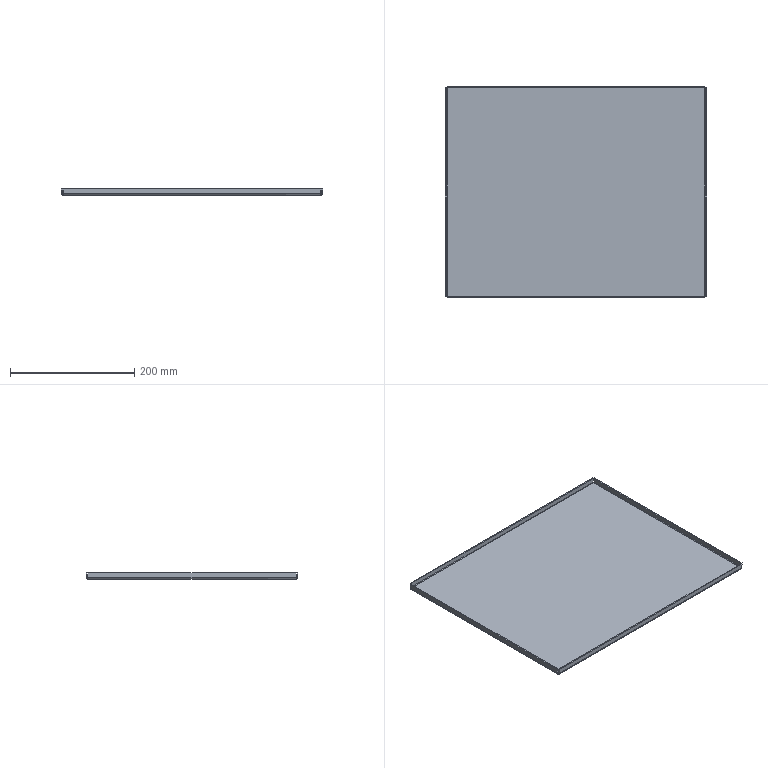Part | SolidWorks | features BaseBody 1 | 1 solid | 38 faces | box 420 x 340 x 10 mm | volume 307281 mm3 | plane 22 | cylinder 8 | spline 8 | commonest cylinder face diameters 1.473 x4 5.473 x4
STEP:
#1=CARTESIAN_POINT('',(-207.263,-167.263,-2.));
#2=VERTEX_POINT('',#1);
#3=CARTESIAN_POINT('',(-207.263,167.263,-2.));
#4=VERTEX_POINT('',#3);
#5=CARTESIAN_POINT('',(-207.263,0.,-2.));
#6=DIRECTION('',(0.,1.,0.));
#7=VECTOR('',#6,1000.);
#8=LINE('',#5,#7);
#9=EDGE_CURVE('',#2,#4,#8,.T.);
#10=ORIENTED_EDGE('',*,*,#9,.T.);
#11=CARTESIAN_POINT('',(207.263,167.263,-2.));
#12=VERTEX_POINT('',#11);
#13=CARTESIAN_POINT('',(0.,167.263,-2.));
#14=DIRECTION('',(1.,0.,0.));
#15=VECTOR('',#14,1000.);
#16=LINE('',#13,#15);
#17=EDGE_CURVE('',#4,#12,#16,.T.);
#18=ORIENTED_EDGE('',*,*,#17,.T.);
#19=CARTESIAN_POINT('',(207.263,-167.263,-2.));
#20=VERTEX_POINT('',#19);
#21=CARTESIAN_POINT('',(207.263,0.,-2.));
#22=DIRECTION('',(0.,-1.,0.));
#23=VECTOR('',#22,1000.);
#24=LINE('',#21,#23);
#25=EDGE_CURVE('',#12,#20,#24,.T.);
#26=ORIENTED_EDGE('',*,*,#25,.T.);
#27=CARTESIAN_POINT('',(0.,-167.263,-2.));
#28=DIRECTION('',(-1.,0.,0.));
#29=VECTOR('',#28,1000.);
#30=LINE('',#27,#29);
#31=EDGE_CURVE('',#20,#2,#30,.T.);
#32=ORIENTED_EDGE('',*,*,#31,.T.);
#33=EDGE_LOOP('',(#10,#18,#26,#32));
#34=FACE_OUTER_BOUND('',#33,.T.);
#35=CARTESIAN_POINT('',(207.263,-167.263,-2.));
#36=DIRECTION('',(0.,0.,-1.));
#37=DIRECTION('',(-1.,0.,0.));
#38=AXIS2_PLACEMENT_3D('',#35,#36,#37);
#39=PLANE('',#38);
#40=ADVANCED_FACE('',(#34),#39,.T.);
#41=CARTESIAN_POINT('',(-207.293,170.,0.7366));
#42=VERTEX_POINT('',#41);
#43=CARTESIAN_POINT('',(-207.293,170.,0.7366));
#44=CARTESIAN_POINT('',(-207.29,170.,0.3784));
#45=CARTESIAN_POINT('',(-207.288,169.929,0.0203));
#46=CARTESIAN_POINT('',(-207.283,169.655,-0.6416));
#47=CARTESIAN_POINT('',(-207.281,169.452,-0.9452));
#48=CARTESIAN_POINT('',(-207.276,168.945,-1.452));
#49=CARTESIAN_POINT('',(-207.273,168.642,-1.655));
#50=CARTESIAN_POINT('',(-207.268,167.98,-1.929));
#51=CARTESIAN_POINT('',(-207.266,167.622,-2.));
#52=CARTESIAN_POINT('',(-207.263,167.263,-2.));
#53=B_SPLINE_CURVE_WITH_KNOTS('',3,(#43,#44,#45,#46,#47,#48,#49,#50,#51,#52),.UNSPECIFIED.,.F.,.F.,(4,2,2,2,4),(0.,0.25,0.5,0.75,1.),.UNSPECIFIED.);
#54=EDGE_CURVE('',#42,#4,#53,.T.);
#55=ORIENTED_EDGE('',*,*,#54,.F.);
#56=CARTESIAN_POINT('',(207.293,170.,0.7366));
#57=VERTEX_POINT('',#56);
#58=CARTESIAN_POINT('',(0.,170.,0.7366));
#59=DIRECTION('',(-1.,0.,0.));
#60=VECTOR('',#59,1000.);
#61=LINE('',#58,#60);
#62=EDGE_CURVE('',#57,#42,#61,.T.);
#63=ORIENTED_EDGE('',*,*,#62,.F.);
#64=CARTESIAN_POINT('',(207.263,167.263,-2.));
#65=CARTESIAN_POINT('',(207.266,167.622,-2.));
#66=CARTESIAN_POINT('',(207.268,167.98,-1.929));
#67=CARTESIAN_POINT('',(207.273,168.642,-1.655));
#68=CARTESIAN_POINT('',(207.276,168.945,-1.452));
#69=CARTESIAN_POINT('',(207.281,169.452,-0.9452));
#70=CARTESIAN_POINT('',(207.283,169.655,-0.6416));
#71=CARTESIAN_POINT('',(207.288,169.929,0.0203));
#72=CARTESIAN_POINT('',(207.29,170.,0.3784));
#73=CARTESIAN_POINT('',(207.293,170.,0.7366));
#74=B_SPLINE_CURVE_WITH_KNOTS('',3,(#64,#65,#66,#67,#68,#69,#70,#71,#72,#73),.UNSPECIFIED.,.F.,.F.,(4,2,2,2,4),(0.,0.25,0.5,0.75,1.),.UNSPECIFIED.);
#75=EDGE_CURVE('',#12,#57,#74,.T.);
#76=ORIENTED_EDGE('',*,*,#75,.F.);
#77=ORIENTED_EDGE('',*,*,#17,.F.);
#78=EDGE_LOOP('',(#55,#63,#76,#77));
#79=FACE_OUTER_BOUND('',#78,.T.);
#80=CARTESIAN_POINT('',(209.78,167.263,0.7366));
#81=DIRECTION('',(-1.,0.,0.));
#82=DIRECTION('',(0.,0.,1.));
#83=AXIS2_PLACEMENT_3D('',#80,#81,#82);
#84=CYLINDRICAL_SURFACE('',#83,2.737);
#85=ADVANCED_FACE('',(#79),#84,.T.);
#86=CARTESIAN_POINT('',(-210.,-167.293,0.7366));
#87=VERTEX_POINT('',#86);
#88=CARTESIAN_POINT('',(-210.,-167.293,0.7366));
#89=CARTESIAN_POINT('',(-210.,-167.29,0.3784));
#90=CARTESIAN_POINT('',(-209.929,-167.288,0.0203));
#91=CARTESIAN_POINT('',(-209.655,-167.283,-0.6416));
#92=CARTESIAN_POINT('',(-209.452,-167.281,-0.9452));
#93=CARTESIAN_POINT('',(-208.945,-167.276,-1.452));
#94=CARTESIAN_POINT('',(-208.642,-167.273,-1.655));
#95=CARTESIAN_POINT('',(-207.98,-167.268,-1.929));
#96=CARTESIAN_POINT('',(-207.622,-167.266,-2.));
#97=CARTESIAN_POINT('',(-207.263,-167.263,-2.));
#98=B_SPLINE_CURVE_WITH_KNOTS('',3,(#88,#89,#90,#91,#92,#93,#94,#95,#96,#97),.UNSPECIFIED.,.F.,.F.,(4,2,2,2,4),(0.,0.25,0.5,0.75,1.),.UNSPECIFIED.);
#99=EDGE_CURVE('',#87,#2,#98,.T.);
#100=ORIENTED_EDGE('',*,*,#99,.F.);
#101=CARTESIAN_POINT('',(-210.,167.293,0.7366));
#102=VERTEX_POINT('',#101);
#103=CARTESIAN_POINT('',(-210.,0.,0.7366));
#104=DIRECTION('',(0.,-1.,0.));
#105=VECTOR('',#104,1000.);
#106=LINE('',#103,#105);
#107=EDGE_CURVE('',#102,#87,#106,.T.);
#108=ORIENTED_EDGE('',*,*,#107,.F.);
#109=CARTESIAN_POINT('',(-207.263,167.263,-2.));
#110=CARTESIAN_POINT('',(-207.622,167.266,-2.));
#111=CARTESIAN_POINT('',(-207.98,167.268,-1.929));
#112=CARTESIAN_POINT('',(-208.642,167.273,-1.655));
#113=CARTESIAN_POINT('',(-208.945,167.276,-1.452));
#114=CARTESIAN_POINT('',(-209.452,167.281,-0.9452));
#115=CARTESIAN_POINT('',(-209.655,167.283,-0.6416));
#116=CARTESIAN_POINT('',(-209.929,167.288,0.0203));
#117=CARTESIAN_POINT('',(-210.,167.29,0.3784));
#118=CARTESIAN_POINT('',(-210.,167.293,0.7366));
#119=B_SPLINE_CURVE_WITH_KNOTS('',3,(#109,#110,#111,#112,#113,#114,#115,#116,#117,#118),.UNSPECIFIED.,.F.,.F.,(4,2,2,2,4),(0.,0.25,0.5,0.75,1.),.UNSPECIFIED.);
#120=EDGE_CURVE('',#4,#102,#119,.T.);
#121=ORIENTED_EDGE('',*,*,#120,.F.);
#122=ORIENTED_EDGE('',*,*,#9,.F.);
#123=EDGE_LOOP('',(#100,#108,#121,#122));
#124=FACE_OUTER_BOUND('',#123,.T.);
#125=CARTESIAN_POINT('',(-207.263,169.3,0.7366));
#126=DIRECTION('',(0.,-1.,0.));
#127=DIRECTION('',(0.,0.,-1.));
#128=AXIS2_PLACEMENT_3D('',#125,#126,#127);
#129=CYLINDRICAL_SURFACE('',#128,2.737);
#130=ADVANCED_FACE('',(#124),#129,.T.);
#131=CARTESIAN_POINT('',(207.293,-170.,0.7366));
#132=VERTEX_POINT('',#131);
#133=CARTESIAN_POINT('',(207.293,-170.,0.7366));
#134=CARTESIAN_POINT('',(207.29,-170.,0.3784));
#135=CARTESIAN_POINT('',(207.288,-169.929,0.0203));
#136=CARTESIAN_POINT('',(207.283,-169.655,-0.6416));
#137=CARTESIAN_POINT('',(207.281,-169.452,-0.9452));
#138=CARTESIAN_POINT('',(207.276,-168.945,-1.452));
#139=CARTESIAN_POINT('',(207.273,-168.642,-1.655));
#140=CARTESIAN_POINT('',(207.268,-167.98,-1.929));
#141=CARTESIAN_POINT('',(207.266,-167.622,-2.));
#142=CARTESIAN_POINT('',(207.263,-167.263,-2.));
#143=B_SPLINE_CURVE_WITH_KNOTS('',3,(#133,#134,#135,#136,#137,#138,#139,#140,#141,#142),.UNSPECIFIED.,.F.,.F.,(4,2,2,2,4),(0.,0.25,0.5,0.75,1.),.UNSPECIFIED.);
#144=EDGE_CURVE('',#132,#20,#143,.T.);
#145=ORIENTED_EDGE('',*,*,#144,.F.);
#146=CARTESIAN_POINT('',(-207.293,-170.,0.7366));
#147=VERTEX_POINT('',#146);
#148=CARTESIAN_POINT('',(0.,-170.,0.7366));
#149=DIRECTION('',(1.,0.,0.));
#150=VECTOR('',#149,1000.);
#151=LINE('',#148,#150);
#152=EDGE_CURVE('',#147,#132,#151,.T.);
#153=ORIENTED_EDGE('',*,*,#152,.F.);
#154=CARTESIAN_POINT('',(-207.263,-167.263,-2.));
#155=CARTESIAN_POINT('',(-207.266,-167.622,-2.));
#156=CARTESIAN_POINT('',(-207.268,-167.98,-1.929));
#157=CARTESIAN_POINT('',(-207.273,-168.642,-1.655));
#158=CARTESIAN_POINT('',(-207.276,-168.945,-1.452));
#159=CARTESIAN_POINT('',(-207.281,-169.452,-0.9452));
#160=CARTESIAN_POINT('',(-207.283,-169.655,-0.6416));
#161=CARTESIAN_POINT('',(-207.288,-169.929,0.0203));
#162=CARTESIAN_POINT('',(-207.29,-170.,0.3784));
#163=CARTESIAN_POINT('',(-207.293,-170.,0.7366));
#164=B_SPLINE_CURVE_WITH_KNOTS('',3,(#154,#155,#156,#157,#158,#159,#160,#161,#162,#163),.UNSPECIFIED.,.F.,.F.,(4,2,2,2,4),(0.,0.25,0.5,0.75,1.),.UNSPECIFIED.);
#165=EDGE_CURVE('',#2,#147,#164,.T.);
#166=ORIENTED_EDGE('',*,*,#165,.F.);
#167=ORIENTED_EDGE('',*,*,#31,.F.);
#168=EDGE_LOOP('',(#145,#153,#166,#167));
#169=FACE_OUTER_BOUND('',#168,.T.);
#170=CARTESIAN_POINT('',(-209.78,-167.263,0.7366));
#171=DIRECTION('',(1.,0.,0.));
#172=DIRECTION('',(0.,0.,-1.));
#173=AXIS2_PLACEMENT_3D('',#170,#171,#172);
#174=CYLINDRICAL_SURFACE('',#173,2.737);
#175=ADVANCED_FACE('',(#169),#174,.T.);
#176=CARTESIAN_POINT('',(210.,167.293,0.7366));
#177=VERTEX_POINT('',#176);
#178=CARTESIAN_POINT('',(210.,167.293,0.7366));
#179=CARTESIAN_POINT('',(210.,167.29,0.3784));
#180=CARTESIAN_POINT('',(209.929,167.288,0.0203));
#181=CARTESIAN_POINT('',(209.655,167.283,-0.6416));
#182=CARTESIAN_POINT('',(209.452,167.281,-0.9452));
#183=CARTESIAN_POINT('',(208.945,167.276,-1.452));
#184=CARTESIAN_POINT('',(208.642,167.273,-1.655));
#185=CARTESIAN_POINT('',(207.98,167.268,-1.929));
#186=CARTESIAN_POINT('',(207.622,167.266,-2.));
#187=CARTESIAN_POINT('',(207.263,167.263,-2.));
#188=B_SPLINE_CURVE_WITH_KNOTS('',3,(#178,#179,#180,#181,#182,#183,#184,#185,#186,#187),.UNSPECIFIED.,.F.,.F.,(4,2,2,2,4),(0.,0.25,0.5,0.75,1.),.UNSPECIFIED.);
#189=EDGE_CURVE('',#177,#12,#188,.T.);
#190=ORIENTED_EDGE('',*,*,#189,.F.);
#191=CARTESIAN_POINT('',(210.,-167.293,0.7366));
#192=VERTEX_POINT('',#191);
#193=CARTESIAN_POINT('',(210.,0.,0.7366));
#194=DIRECTION('',(0.,1.,0.));
#195=VECTOR('',#194,1000.);
#196=LINE('',#193,#195);
#197=EDGE_CURVE('',#192,#177,#196,.T.);
#198=ORIENTED_EDGE('',*,*,#197,.F.);
#199=CARTESIAN_POINT('',(207.263,-167.263,-2.));
#200=CARTESIAN_POINT('',(207.622,-167.266,-2.));
#201=CARTESIAN_POINT('',(207.98,-167.268,-1.929));
#202=CARTESIAN_POINT('',(208.642,-167.273,-1.655));
#203=CARTESIAN_POINT('',(208.945,-167.276,-1.452));
#204=CARTESIAN_POINT('',(209.452,-167.281,-0.9452));
#205=CARTESIAN_POINT('',(209.655,-167.283,-0.6416));
#206=CARTESIAN_POINT('',(209.929,-167.288,0.0203));
#207=CARTESIAN_POINT('',(210.,-167.29,0.3784));
#208=CARTESIAN_POINT('',(210.,-167.293,0.7366));
#209=B_SPLINE_CURVE_WITH_KNOTS('',3,(#199,#200,#201,#202,#203,#204,#205,#206,#207,#208),.UNSPECIFIED.,.F.,.F.,(4,2,2,2,4),(0.,0.25,0.5,0.75,1.),.UNSPECIFIED.);
#210=EDGE_CURVE('',#20,#192,#209,.T.);
#211=ORIENTED_EDGE('',*,*,#210,.F.);
#212=ORIENTED_EDGE('',*,*,#25,.F.);
#213=EDGE_LOOP('',(#190,#198,#211,#212));
#214=FACE_OUTER_BOUND('',#213,.T.);
#215=CARTESIAN_POINT('',(207.263,-169.3,0.7366));
#216=DIRECTION('',(0.,1.,0.));
#217=DIRECTION('',(0.,0.,1.));
#218=AXIS2_PLACEMENT_3D('',#215,#216,#217);
#219=CYLINDRICAL_SURFACE('',#218,2.737);
#220=ADVANCED_FACE('',(#214),#219,.T.);
#221=CARTESIAN_POINT('',(-207.293,168.,0.7366));
#222=VERTEX_POINT('',#221);
#223=CARTESIAN_POINT('',(-207.293,169.,0.7366));
#224=DIRECTION('',(0.,-1.,0.));
#225=VECTOR('',#224,1000.);
#226=LINE('',#223,#225);
#227=EDGE_CURVE('',#42,#222,#226,.T.);
#228=ORIENTED_EDGE('',*,*,#227,.F.);
#229=ORIENTED_EDGE('',*,*,#54,.T.);
#230=CARTESIAN_POINT('',(-207.263,167.263,0.));
#231=VERTEX_POINT('',#230);
#232=CARTESIAN_POINT('',(-207.263,167.263,-1.));
#233=DIRECTION('',(0.,0.,-1.));
#234=VECTOR('',#233,1000.);
#235=LINE('',#232,#234);
#236=EDGE_CURVE('',#231,#4,#235,.T.);
#237=ORIENTED_EDGE('',*,*,#236,.F.);
#238=CARTESIAN_POINT('',(-207.293,168.,0.7366));
#239=CARTESIAN_POINT('',(-207.288,168.,0.5438));
#240=CARTESIAN_POINT('',(-207.283,167.921,0.3521));
#241=CARTESIAN_POINT('',(-207.273,167.648,0.07939));
#242=CARTESIAN_POINT('',(-207.268,167.456,0.));
#243=CARTESIAN_POINT('',(-207.263,167.263,0.));
#244=B_SPLINE_CURVE_WITH_KNOTS('',3,(#238,#239,#240,#241,#242,#243),.UNSPECIFIED.,.F.,.F.,(4,2,4),(0.,0.5,1.),.UNSPECIFIED.);
#245=EDGE_CURVE('',#222,#231,#244,.T.);
#246=ORIENTED_EDGE('',*,*,#245,.F.);
#247=EDGE_LOOP('',(#228,#229,#237,#246));
#248=FACE_OUTER_BOUND('',#247,.T.);
#249=CARTESIAN_POINT('',(-207.293,170.012,0.7366));
#250=CARTESIAN_POINT('',(-207.29,170.012,0.3767));
#251=CARTESIAN_POINT('',(-207.288,169.941,0.01711));
#252=CARTESIAN_POINT('',(-207.283,169.665,-0.6477));
#253=CARTESIAN_POINT('',(-207.281,169.462,-0.9527));
#254=CARTESIAN_POINT('',(-207.276,168.953,-1.462));
#255=CARTESIAN_POINT('',(-207.273,168.648,-1.665));
#256=CARTESIAN_POINT('',(-207.268,167.983,-1.941));
#257=CARTESIAN_POINT('',(-207.266,167.623,-2.012));
#258=CARTESIAN_POINT('',(-207.263,167.263,-2.012));
#259=CARTESIAN_POINT('',(-207.293,170.,0.7366));
#260=CARTESIAN_POINT('',(-207.29,170.,0.3783));
#261=CARTESIAN_POINT('',(-207.288,169.929,0.0203));
#262=CARTESIAN_POINT('',(-207.283,169.655,-0.6416));
#263=CARTESIAN_POINT('',(-207.281,169.452,-0.9452));
#264=CARTESIAN_POINT('',(-207.276,168.945,-1.452));
#265=CARTESIAN_POINT('',(-207.273,168.642,-1.655));
#266=CARTESIAN_POINT('',(-207.268,167.98,-1.929));
#267=CARTESIAN_POINT('',(-207.266,167.622,-2.));
#268=CARTESIAN_POINT('',(-207.263,167.263,-2.));
#269=CARTESIAN_POINT('',(-207.293,168.,0.7366));
#270=CARTESIAN_POINT('',(-207.29,168.,0.6402));
#271=CARTESIAN_POINT('',(-207.288,167.981,0.5438));
#272=CARTESIAN_POINT('',(-207.283,167.907,0.3656));
#273=CARTESIAN_POINT('',(-207.281,167.852,0.2839));
#274=CARTESIAN_POINT('',(-207.276,167.716,0.1476));
#275=CARTESIAN_POINT('',(-207.273,167.634,0.09297));
#276=CARTESIAN_POINT('',(-207.268,167.456,0.01917));
#277=CARTESIAN_POINT('',(-207.266,167.36,0.));
#278=CARTESIAN_POINT('',(-207.263,167.263,0.));
#279=CARTESIAN_POINT('',(-207.293,167.988,0.7366));
#280=CARTESIAN_POINT('',(-207.29,167.988,0.6417));
#281=CARTESIAN_POINT('',(-207.288,167.969,0.5469));
#282=CARTESIAN_POINT('',(-207.283,167.897,0.3717));
#283=CARTESIAN_POINT('',(-207.281,167.843,0.2913));
#284=CARTESIAN_POINT('',(-207.276,167.709,0.1572));
#285=CARTESIAN_POINT('',(-207.273,167.628,0.1035));
#286=CARTESIAN_POINT('',(-207.268,167.453,0.03088));
#287=CARTESIAN_POINT('',(-207.266,167.358,0.01202));
#288=CARTESIAN_POINT('',(-207.263,167.263,0.01202));
#289=B_SPLINE_SURFACE_WITH_KNOTS('',1,3,((#249,#250,#251,#252,#253,#254,#255,#256,#257,#258),(#259,#260,#261,#262,#263,#264,#265,#266,#267,#268),(#269,#270,#271,#272,#273,#274,#275,#276,#277,#278),(#279,#280,#281,#282,#283,#284,#285,#286,#287,#288)),.UNSPECIFIED.,.F.,.F.,.F.,(2,1,1,2),(4,2,2,2,4),(-0.006096,0.,1.,1.006),(0.,0.25,0.5,0.75,1.),.UNSPECIFIED.);
#290=ADVANCED_FACE('',(#248),#289,.F.);
#291=CARTESIAN_POINT('',(-207.293,170.,8.));
#292=VERTEX_POINT('',#291);
#293=CARTESIAN_POINT('',(-207.293,170.,4.368));
#294=DIRECTION('',(0.,0.,-1.));
#295=VECTOR('',#294,1000.);
#296=LINE('',#293,#295);
#297=EDGE_CURVE('',#292,#42,#296,.T.);
#298=ORIENTED_EDGE('',*,*,#297,.F.);
#299=CARTESIAN_POINT('',(207.293,170.,8.));
#300=VERTEX_POINT('',#299);
#301=CARTESIAN_POINT('',(0.,170.,8.));
#302=DIRECTION('',(-1.,0.,0.));
#303=VECTOR('',#302,1000.);
#304=LINE('',#301,#303);
#305=EDGE_CURVE('',#300,#292,#304,.T.);
#306=ORIENTED_EDGE('',*,*,#305,.F.);
#307=CARTESIAN_POINT('',(207.293,170.,4.368));
#308=DIRECTION('',(0.,0.,1.));
#309=VECTOR('',#308,1000.);
#310=LINE('',#307,#309);
#311=EDGE_CURVE('',#57,#300,#310,.T.);
#312=ORIENTED_EDGE('',*,*,#311,.F.);
#313=ORIENTED_EDGE('',*,*,#62,.T.);
#314=EDGE_LOOP('',(#298,#306,#312,#313));
#315=FACE_OUTER_BOUND('',#314,.T.);
#316=CARTESIAN_POINT('',(-207.293,170.,8.));
#317=DIRECTION('',(0.,-1.,0.));
#318=DIRECTION('',(0.,0.,-1.));
#319=AXIS2_PLACEMENT_3D('',#316,#317,#318);
#320=PLANE('',#319);
#321=ADVANCED_FACE('',(#315),#320,.F.);
#322=CARTESIAN_POINT('',(207.263,167.263,0.));
#323=VERTEX_POINT('',#322);
#324=CARTESIAN_POINT('',(207.293,168.,0.7366));
#325=VERTEX_POINT('',#324);
#326=CARTESIAN_POINT('',(207.263,167.263,0.));
#327=CARTESIAN_POINT('',(207.268,167.456,0.));
#328=CARTESIAN_POINT('',(207.273,167.648,0.07939));
#329=CARTESIAN_POINT('',(207.283,167.921,0.3521));
#330=CARTESIAN_POINT('',(207.288,168.,0.5438));
#331=CARTESIAN_POINT('',(207.293,168.,0.7366));
#332=B_SPLINE_CURVE_WITH_KNOTS('',3,(#326,#327,#328,#329,#330,#331),.UNSPECIFIED.,.F.,.F.,(4,2,4),(0.,0.5,1.),.UNSPECIFIED.);
#333=EDGE_CURVE('',#323,#325,#332,.T.);
#334=ORIENTED_EDGE('',*,*,#333,.F.);
#335=CARTESIAN_POINT('',(207.263,167.263,-1.));
#336=DIRECTION('',(0.,0.,1.));
#337=VECTOR('',#336,1000.);
#338=LINE('',#335,#337);
#339=EDGE_CURVE('',#12,#323,#338,.T.);
#340=ORIENTED_EDGE('',*,*,#339,.F.);
#341=ORIENTED_EDGE('',*,*,#75,.T.);
#342=CARTESIAN_POINT('',(207.293,169.,0.7366));
#343=DIRECTION('',(0.,1.,0.));
#344=VECTOR('',#343,1000.);
#345=LINE('',#342,#344);
#346=EDGE_CURVE('',#325,#57,#345,.T.);
#347=ORIENTED_EDGE('',*,*,#346,.F.);
#348=EDGE_LOOP('',(#334,#340,#341,#347));
#349=FACE_OUTER_BOUND('',#348,.T.);
#350=CARTESIAN_POINT('',(207.263,167.263,-2.012));
#351=CARTESIAN_POINT('',(207.266,167.623,-2.012));
#352=CARTESIAN_POINT('',(207.268,167.983,-1.941));
#353=CARTESIAN_POINT('',(207.273,168.648,-1.665));
#354=CARTESIAN_POINT('',(207.276,168.953,-1.462));
#355=CARTESIAN_POINT('',(207.281,169.462,-0.9527));
#356=CARTESIAN_POINT('',(207.283,169.665,-0.6477));
#357=CARTESIAN_POINT('',(207.288,169.941,0.01711));
#358=CARTESIAN_POINT('',(207.29,170.012,0.3767));
#359=CARTESIAN_POINT('',(207.293,170.012,0.7366));
#360=CARTESIAN_POINT('',(207.263,167.263,-2.));
#361=CARTESIAN_POINT('',(207.266,167.622,-2.));
#362=CARTESIAN_POINT('',(207.268,167.98,-1.929));
#363=CARTESIAN_POINT('',(207.273,168.642,-1.655));
#364=CARTESIAN_POINT('',(207.276,168.945,-1.452));
#365=CARTESIAN_POINT('',(207.281,169.452,-0.9452));
#366=CARTESIAN_POINT('',(207.283,169.655,-0.6416));
#367=CARTESIAN_POINT('',(207.288,169.929,0.0203));
#368=CARTESIAN_POINT('',(207.29,170.,0.3783));
#369=CARTESIAN_POINT('',(207.293,170.,0.7366));
#370=CARTESIAN_POINT('',(207.263,167.263,0.));
#371=CARTESIAN_POINT('',(207.266,167.36,0.));
#372=CARTESIAN_POINT('',(207.268,167.456,0.01917));
#373=CARTESIAN_POINT('',(207.273,167.634,0.09297));
#374=CARTESIAN_POINT('',(207.276,167.716,0.1476));
#375=CARTESIAN_POINT('',(207.281,167.852,0.2839));
#376=CARTESIAN_POINT('',(207.283,167.907,0.3656));
#377=CARTESIAN_POINT('',(207.288,167.981,0.5438));
#378=CARTESIAN_POINT('',(207.29,168.,0.6402));
#379=CARTESIAN_POINT('',(207.293,168.,0.7366));
#380=CARTESIAN_POINT('',(207.263,167.263,0.01202));
#381=CARTESIAN_POINT('',(207.266,167.358,0.01202));
#382=CARTESIAN_POINT('',(207.268,167.453,0.03088));
#383=CARTESIAN_POINT('',(207.273,167.628,0.1035));
#384=CARTESIAN_POINT('',(207.276,167.709,0.1572));
#385=CARTESIAN_POINT('',(207.281,167.843,0.2913));
#386=CARTESIAN_POINT('',(207.283,167.897,0.3717));
#387=CARTESIAN_POINT('',(207.288,167.969,0.5469));
#388=CARTESIAN_POINT('',(207.29,167.988,0.6417));
#389=CARTESIAN_POINT('',(207.293,167.988,0.7366));
#390=B_SPLINE_SURFACE_WITH_KNOTS('',1,3,((#350,#351,#352,#353,#354,#355,#356,#357,#358,#359),(#360,#361,#362,#363,#364,#365,#366,#367,#368,#369),(#370,#371,#372,#373,#374,#375,#376,#377,#378,#379),(#380,#381,#382,#383,#384,#385,#386,#387,#388,#389)),.UNSPECIFIED.,.F.,.F.,.F.,(2,1,1,2),(4,2,2,2,4),(-0.006096,0.,1.,1.006),(0.,0.25,0.5,0.75,1.),.UNSPECIFIED.);
#391=ADVANCED_FACE('',(#349),#390,.F.);
#392=CARTESIAN_POINT('',(-208.,-167.293,0.7366));
#393=VERTEX_POINT('',#392);
#394=CARTESIAN_POINT('',(-209.,-167.293,0.7366));
#395=DIRECTION('',(1.,0.,0.));
#396=VECTOR('',#395,1000.);
#397=LINE('',#394,#396);
#398=EDGE_CURVE('',#87,#393,#397,.T.);
#399=ORIENTED_EDGE('',*,*,#398,.F.);
#400=ORIENTED_EDGE('',*,*,#99,.T.);
#401=CARTESIAN_POINT('',(-207.263,-167.263,0.));
#402=VERTEX_POINT('',#401);
#403=CARTESIAN_POINT('',(-207.263,-167.263,-1.));
#404=DIRECTION('',(0.,0.,-1.));
#405=VECTOR('',#404,1000.);
#406=LINE('',#403,#405);
#407=EDGE_CURVE('',#402,#2,#406,.T.);
#408=ORIENTED_EDGE('',*,*,#407,.F.);
#409=CARTESIAN_POINT('',(-208.,-167.293,0.7366));
#410=CARTESIAN_POINT('',(-208.,-167.288,0.5438));
#411=CARTESIAN_POINT('',(-207.921,-167.283,0.3521));
#412=CARTESIAN_POINT('',(-207.648,-167.273,0.07939));
#413=CARTESIAN_POINT('',(-207.456,-167.268,0.));
#414=CARTESIAN_POINT('',(-207.263,-167.263,0.));
#415=B_SPLINE_CURVE_WITH_KNOTS('',3,(#409,#410,#411,#412,#413,#414),.UNSPECIFIED.,.F.,.F.,(4,2,4),(0.,0.5,1.),.UNSPECIFIED.);
#416=EDGE_CURVE('',#393,#402,#415,.T.);
#417=ORIENTED_EDGE('',*,*,#416,.F.);
#418=EDGE_LOOP('',(#399,#400,#408,#417));
#419=FACE_OUTER_BOUND('',#418,.T.);
#420=CARTESIAN_POINT('',(-210.012,-167.293,0.7366));
#421=CARTESIAN_POINT('',(-210.012,-167.29,0.3767));
#422=CARTESIAN_POINT('',(-209.941,-167.288,0.01711));
#423=CARTESIAN_POINT('',(-209.665,-167.283,-0.6477));
#424=CARTESIAN_POINT('',(-209.462,-167.281,-0.9527));
#425=CARTESIAN_POINT('',(-208.953,-167.276,-1.462));
#426=CARTESIAN_POINT('',(-208.648,-167.273,-1.665));
#427=CARTESIAN_POINT('',(-207.983,-167.268,-1.941));
#428=CARTESIAN_POINT('',(-207.623,-167.266,-2.012));
#429=CARTESIAN_POINT('',(-207.263,-167.263,-2.012));
#430=CARTESIAN_POINT('',(-210.,-167.293,0.7366));
#431=CARTESIAN_POINT('',(-210.,-167.29,0.3783));
#432=CARTESIAN_POINT('',(-209.929,-167.288,0.0203));
#433=CARTESIAN_POINT('',(-209.655,-167.283,-0.6416));
#434=CARTESIAN_POINT('',(-209.452,-167.281,-0.9452));
#435=CARTESIAN_POINT('',(-208.945,-167.276,-1.452));
#436=CARTESIAN_POINT('',(-208.642,-167.273,-1.655));
#437=CARTESIAN_POINT('',(-207.98,-167.268,-1.929));
#438=CARTESIAN_POINT('',(-207.622,-167.266,-2.));
#439=CARTESIAN_POINT('',(-207.263,-167.263,-2.));
#440=CARTESIAN_POINT('',(-208.,-167.293,0.7366));
#441=CARTESIAN_POINT('',(-208.,-167.29,0.6402));
#442=CARTESIAN_POINT('',(-207.981,-167.288,0.5438));
#443=CARTESIAN_POINT('',(-207.907,-167.283,0.3656));
#444=CARTESIAN_POINT('',(-207.852,-167.281,0.2839));
#445=CARTESIAN_POINT('',(-207.716,-167.276,0.1476));
#446=CARTESIAN_POINT('',(-207.634,-167.273,0.09297));
#447=CARTESIAN_POINT('',(-207.456,-167.268,0.01917));
#448=CARTESIAN_POINT('',(-207.36,-167.266,0.));
#449=CARTESIAN_POINT('',(-207.263,-167.263,0.));
#450=CARTESIAN_POINT('',(-207.988,-167.293,0.7366));
#451=CARTESIAN_POINT('',(-207.988,-167.29,0.6417));
#452=CARTESIAN_POINT('',(-207.969,-167.288,0.5469));
#453=CARTESIAN_POINT('',(-207.897,-167.283,0.3717));
#454=CARTESIAN_POINT('',(-207.843,-167.281,0.2913));
#455=CARTESIAN_POINT('',(-207.709,-167.276,0.1572));
#456=CARTESIAN_POINT('',(-207.628,-167.273,0.1035));
#457=CARTESIAN_POINT('',(-207.453,-167.268,0.03088));
#458=CARTESIAN_POINT('',(-207.358,-167.266,0.01202));
#459=CARTESIAN_POINT('',(-207.263,-167.263,0.01202));
#460=B_SPLINE_SURFACE_WITH_KNOTS('',1,3,((#420,#421,#422,#423,#424,#425,#426,#427,#428,#429),(#430,#431,#432,#433,#434,#435,#436,#437,#438,#439),(#440,#441,#442,#443,#444,#445,#446,#447,#448,#449),(#450,#451,#452,#453,#454,#455,#456,#457,#458,#459)),.UNSPECIFIED.,.F.,.F.,.F.,(2,1,1,2),(4,2,2,2,4),(-0.006096,0.,1.,1.006),(0.,0.25,0.5,0.75,1.),.UNSPECIFIED.);
#461=ADVANCED_FACE('',(#419),#460,.F.);
#462=CARTESIAN_POINT('',(-210.,-167.293,8.));
#463=VERTEX_POINT('',#462);
#464=CARTESIAN_POINT('',(-210.,-167.293,4.368));
#465=DIRECTION('',(0.,0.,-1.));
#466=VECTOR('',#465,1000.);
#467=LINE('',#464,#466);
#468=EDGE_CURVE('',#463,#87,#467,.T.);
#469=ORIENTED_EDGE('',*,*,#468,.F.);
#470=CARTESIAN_POINT('',(-210.,167.293,8.));
#471=VERTEX_POINT('',#470);
#472=CARTESIAN_POINT('',(-210.,0.,8.));
#473=DIRECTION('',(0.,-1.,0.));
#474=VECTOR('',#473,1000.);
#475=LINE('',#472,#474);
#476=EDGE_CURVE('',#471,#463,#475,.T.);
#477=ORIENTED_EDGE('',*,*,#476,.F.);
#478=CARTESIAN_POINT('',(-210.,167.293,4.368));
#479=DIRECTION('',(0.,0.,1.));
#480=VECTOR('',#479,1000.);
#481=LINE('',#478,#480);
#482=EDGE_CURVE('',#102,#471,#481,.T.);
#483=ORIENTED_EDGE('',*,*,#482,.F.);
#484=ORIENTED_EDGE('',*,*,#107,.T.);
#485=EDGE_LOOP('',(#469,#477,#483,#484));
#486=FACE_OUTER_BOUND('',#485,.T.);
#487=CARTESIAN_POINT('',(-210.,-167.293,8.));
#488=DIRECTION('',(1.,0.,0.));
#489=DIRECTION('',(0.,0.,-1.));
#490=AXIS2_PLACEMENT_3D('',#487,#488,#489);
#491=PLANE('',#490);
#492=ADVANCED_FACE('',(#486),#491,.F.);
#493=CARTESIAN_POINT('',(-208.,167.293,0.7366));
#494=VERTEX_POINT('',#493);
#495=CARTESIAN_POINT('',(-207.263,167.263,0.));
#496=CARTESIAN_POINT('',(-207.456,167.268,0.));
#497=CARTESIAN_POINT('',(-207.648,167.273,0.07939));
#498=CARTESIAN_POINT('',(-207.921,167.283,0.3521));
#499=CARTESIAN_POINT('',(-208.,167.288,0.5438));
#500=CARTESIAN_POINT('',(-208.,167.293,0.7366));
#501=B_SPLINE_CURVE_WITH_KNOTS('',3,(#495,#496,#497,#498,#499,#500),.UNSPECIFIED.,.F.,.F.,(4,2,4),(0.,0.5,1.),.UNSPECIFIED.);
#502=EDGE_CURVE('',#231,#494,#501,.T.);
#503=ORIENTED_EDGE('',*,*,#502,.F.);
#504=ORIENTED_EDGE('',*,*,#236,.T.);
#505=ORIENTED_EDGE('',*,*,#120,.T.);
#506=CARTESIAN_POINT('',(-209.,167.293,0.7366));
#507=DIRECTION('',(-1.,0.,0.));
#508=VECTOR('',#507,1000.);
#509=LINE('',#506,#508);
#510=EDGE_CURVE('',#494,#102,#509,.T.);
#511=ORIENTED_EDGE('',*,*,#510,.F.);
#512=EDGE_LOOP('',(#503,#504,#505,#511));
#513=FACE_OUTER_BOUND('',#512,.T.);
#514=CARTESIAN_POINT('',(-207.263,167.263,-2.012));
#515=CARTESIAN_POINT('',(-207.623,167.266,-2.012));
#516=CARTESIAN_POINT('',(-207.983,167.268,-1.941));
#517=CARTESIAN_POINT('',(-208.648,167.273,-1.665));
#518=CARTESIAN_POINT('',(-208.953,167.276,-1.462));
#519=CARTESIAN_POINT('',(-209.462,167.281,-0.9527));
#520=CARTESIAN_POINT('',(-209.665,167.283,-0.6477));
#521=CARTESIAN_POINT('',(-209.941,167.288,0.01711));
#522=CARTESIAN_POINT('',(-210.012,167.29,0.3767));
#523=CARTESIAN_POINT('',(-210.012,167.293,0.7366));
#524=CARTESIAN_POINT('',(-207.263,167.263,-2.));
#525=CARTESIAN_POINT('',(-207.622,167.266,-2.));
#526=CARTESIAN_POINT('',(-207.98,167.268,-1.929));
#527=CARTESIAN_POINT('',(-208.642,167.273,-1.655));
#528=CARTESIAN_POINT('',(-208.945,167.276,-1.452));
#529=CARTESIAN_POINT('',(-209.452,167.281,-0.9452));
#530=CARTESIAN_POINT('',(-209.655,167.283,-0.6416));
#531=CARTESIAN_POINT('',(-209.929,167.288,0.0203));
#532=CARTESIAN_POINT('',(-210.,167.29,0.3783));
#533=CARTESIAN_POINT('',(-210.,167.293,0.7366));
#534=CARTESIAN_POINT('',(-207.263,167.263,0.));
#535=CARTESIAN_POINT('',(-207.36,167.266,0.));
#536=CARTESIAN_POINT('',(-207.456,167.268,0.01917));
#537=CARTESIAN_POINT('',(-207.634,167.273,0.09297));
#538=CARTESIAN_POINT('',(-207.716,167.276,0.1476));
#539=CARTESIAN_POINT('',(-207.852,167.281,0.2839));
#540=CARTESIAN_POINT('',(-207.907,167.283,0.3656));
#541=CARTESIAN_POINT('',(-207.981,167.288,0.5438));
#542=CARTESIAN_POINT('',(-208.,167.29,0.6402));
#543=CARTESIAN_POINT('',(-208.,167.293,0.7366));
#544=CARTESIAN_POINT('',(-207.263,167.263,0.01202));
#545=CARTESIAN_POINT('',(-207.358,167.266,0.01202));
#546=CARTESIAN_POINT('',(-207.453,167.268,0.03088));
#547=CARTESIAN_POINT('',(-207.628,167.273,0.1035));
#548=CARTESIAN_POINT('',(-207.709,167.276,0.1572));
#549=CARTESIAN_POINT('',(-207.843,167.281,0.2913));
#550=CARTESIAN_POINT('',(-207.897,167.283,0.3717));
#551=CARTESIAN_POINT('',(-207.969,167.288,0.5469));
#552=CARTESIAN_POINT('',(-207.988,167.29,0.6417));
#553=CARTESIAN_POINT('',(-207.988,167.293,0.7366));
#554=B_SPLINE_SURFACE_WITH_KNOTS('',1,3,((#514,#515,#516,#517,#518,#519,#520,#521,#522,#523),(#524,#525,#526,#527,#528,#529,#530,#531,#532,#533),(#534,#535,#536,#537,#538,#539,#540,#541,#542,#543),(#544,#545,#546,#547,#548,#549,#550,#551,#552,#553)),.UNSPECIFIED.,.F.,.F.,.F.,(2,1,1,2),(4,2,2,2,4),(-0.006096,0.,1.,1.006),(0.,0.25,0.5,0.75,1.),.UNSPECIFIED.);
#555=ADVANCED_FACE('',(#513),#554,.F.);
#556=CARTESIAN_POINT('',(207.293,-168.,0.7366));
#557=VERTEX_POINT('',#556);
#558=CARTESIAN_POINT('',(207.293,-169.,0.7366));
#559=DIRECTION('',(0.,1.,0.));
#560=VECTOR('',#559,1000.);
#561=LINE('',#558,#560);
#562=EDGE_CURVE('',#132,#557,#561,.T.);
#563=ORIENTED_EDGE('',*,*,#562,.F.);
#564=ORIENTED_EDGE('',*,*,#144,.T.);
#565=CARTESIAN_POINT('',(207.263,-167.263,0.));
#566=VERTEX_POINT('',#565);
#567=CARTESIAN_POINT('',(207.263,-167.263,-1.));
#568=DIRECTION('',(0.,0.,-1.));
#569=VECTOR('',#568,1000.);
#570=LINE('',#567,#569);
#571=EDGE_CURVE('',#566,#20,#570,.T.);
#572=ORIENTED_EDGE('',*,*,#571,.F.);
#573=CARTESIAN_POINT('',(207.293,-168.,0.7366));
#574=CARTESIAN_POINT('',(207.288,-168.,0.5438));
#575=CARTESIAN_POINT('',(207.283,-167.921,0.3521));
#576=CARTESIAN_POINT('',(207.273,-167.648,0.07939));
#577=CARTESIAN_POINT('',(207.268,-167.456,0.));
#578=CARTESIAN_POINT('',(207.263,-167.263,0.));
#579=B_SPLINE_CURVE_WITH_KNOTS('',3,(#573,#574,#575,#576,#577,#578),.UNSPECIFIED.,.F.,.F.,(4,2,4),(0.,0.5,1.),.UNSPECIFIED.);
#580=EDGE_CURVE('',#557,#566,#579,.T.);
#581=ORIENTED_EDGE('',*,*,#580,.F.);
#582=EDGE_LOOP('',(#563,#564,#572,#581));
#583=FACE_OUTER_BOUND('',#582,.T.);
#584=CARTESIAN_POINT('',(207.293,-170.012,0.7366));
#585=CARTESIAN_POINT('',(207.29,-170.012,0.3767));
#586=CARTESIAN_POINT('',(207.288,-169.941,0.01711));
#587=CARTESIAN_POINT('',(207.283,-169.665,-0.6477));
#588=CARTESIAN_POINT('',(207.281,-169.462,-0.9527));
#589=CARTESIAN_POINT('',(207.276,-168.953,-1.462));
#590=CARTESIAN_POINT('',(207.273,-168.648,-1.665));
#591=CARTESIAN_POINT('',(207.268,-167.983,-1.941));
#592=CARTESIAN_POINT('',(207.266,-167.623,-2.012));
#593=CARTESIAN_POINT('',(207.263,-167.263,-2.012));
#594=CARTESIAN_POINT('',(207.293,-170.,0.7366));
#595=CARTESIAN_POINT('',(207.29,-170.,0.3783));
#596=CARTESIAN_POINT('',(207.288,-169.929,0.0203));
#597=CARTESIAN_POINT('',(207.283,-169.655,-0.6416));
#598=CARTESIAN_POINT('',(207.281,-169.452,-0.9452));
#599=CARTESIAN_POINT('',(207.276,-168.945,-1.452));
#600=CARTESIAN_POINT('',(207.273,-168.642,-1.655));
#601=CARTESIAN_POINT('',(207.268,-167.98,-1.929));
#602=CARTESIAN_POINT('',(207.266,-167.622,-2.));
#603=CARTESIAN_POINT('',(207.263,-167.263,-2.));
#604=CARTESIAN_POINT('',(207.293,-168.,0.7366));
#605=CARTESIAN_POINT('',(207.29,-168.,0.6402));
#606=CARTESIAN_POINT('',(207.288,-167.981,0.5438));
#607=CARTESIAN_POINT('',(207.283,-167.907,0.3656));
#608=CARTESIAN_POINT('',(207.281,-167.852,0.2839));
#609=CARTESIAN_POINT('',(207.276,-167.716,0.1476));
#610=CARTESIAN_POINT('',(207.273,-167.634,0.09297));
#611=CARTESIAN_POINT('',(207.268,-167.456,0.01917));
#612=CARTESIAN_POINT('',(207.266,-167.36,0.));
#613=CARTESIAN_POINT('',(207.263,-167.263,0.));
#614=CARTESIAN_POINT('',(207.293,-167.988,0.7366));
#615=CARTESIAN_POINT('',(207.29,-167.988,0.6417));
#616=CARTESIAN_POINT('',(207.288,-167.969,0.5469));
#617=CARTESIAN_POINT('',(207.283,-167.897,0.3717));
#618=CARTESIAN_POINT('',(207.281,-167.843,0.2913));
#619=CARTESIAN_POINT('',(207.276,-167.709,0.1572));
#620=CARTESIAN_POINT('',(207.273,-167.628,0.1035));
#621=CARTESIAN_POINT('',(207.268,-167.453,0.03088));
#622=CARTESIAN_POINT('',(207.266,-167.358,0.01202));
#623=CARTESIAN_POINT('',(207.263,-167.263,0.01202));
#624=B_SPLINE_SURFACE_WITH_KNOTS('',1,3,((#584,#585,#586,#587,#588,#589,#590,#591,#592,#593),(#594,#595,#596,#597,#598,#599,#600,#601,#602,#603),(#604,#605,#606,#607,#608,#609,#610,#611,#612,#613),(#614,#615,#616,#617,#618,#619,#620,#621,#622,#623)),.UNSPECIFIED.,.F.,.F.,.F.,(2,1,1,2),(4,2,2,2,4),(-0.006096,0.,1.,1.006),(0.,0.25,0.5,0.75,1.),.UNSPECIFIED.);
#625=ADVANCED_FACE('',(#583),#624,.F.);
#626=CARTESIAN_POINT('',(207.293,-170.,8.));
#627=VERTEX_POINT('',#626);
#628=CARTESIAN_POINT('',(207.293,-170.,4.368));
#629=DIRECTION('',(0.,0.,-1.));
#630=VECTOR('',#629,1000.);
#631=LINE('',#628,#630);
#632=EDGE_CURVE('',#627,#132,#631,.T.);
#633=ORIENTED_EDGE('',*,*,#632,.F.);
#634=CARTESIAN_POINT('',(-207.293,-170.,8.));
#635=VERTEX_POINT('',#634);
#636=CARTESIAN_POINT('',(0.,-170.,8.));
#637=DIRECTION('',(1.,0.,0.));
#638=VECTOR('',#637,1000.);
#639=LINE('',#636,#638);
#640=EDGE_CURVE('',#635,#627,#639,.T.);
#641=ORIENTED_EDGE('',*,*,#640,.F.);
#642=CARTESIAN_POINT('',(-207.293,-170.,4.368));
#643=DIRECTION('',(0.,0.,1.));
#644=VECTOR('',#643,1000.);
#645=LINE('',#642,#644);
#646=EDGE_CURVE('',#147,#635,#645,.T.);
#647=ORIENTED_EDGE('',*,*,#646,.F.);
#648=ORIENTED_EDGE('',*,*,#152,.T.);
#649=EDGE_LOOP('',(#633,#641,#647,#648));
#650=FACE_OUTER_BOUND('',#649,.T.);
#651=CARTESIAN_POINT('',(-207.293,-170.,0.7366));
#652=DIRECTION('',(0.,1.,0.));
#653=DIRECTION('',(0.,0.,1.));
#654=AXIS2_PLACEMENT_3D('',#651,#652,#653);
#655=PLANE('',#654);
#656=ADVANCED_FACE('',(#650),#655,.F.);
#657=CARTESIAN_POINT('',(-207.293,-168.,0.7366));
#658=VERTEX_POINT('',#657);
#659=CARTESIAN_POINT('',(-207.263,-167.263,0.));
#660=CARTESIAN_POINT('',(-207.268,-167.456,0.));
#661=CARTESIAN_POINT('',(-207.273,-167.648,0.07939));
#662=CARTESIAN_POINT('',(-207.283,-167.921,0.3521));
#663=CARTESIAN_POINT('',(-207.288,-168.,0.5438));
#664=CARTESIAN_POINT('',(-207.293,-168.,0.7366));
#665=B_SPLINE_CURVE_WITH_KNOTS('',3,(#659,#660,#661,#662,#663,#664),.UNSPECIFIED.,.F.,.F.,(4,2,4),(0.,0.5,1.),.UNSPECIFIED.);
#666=EDGE_CURVE('',#402,#658,#665,.T.);
#667=ORIENTED_EDGE('',*,*,#666,.F.);
#668=ORIENTED_EDGE('',*,*,#407,.T.);
#669=ORIENTED_EDGE('',*,*,#165,.T.);
#670=CARTESIAN_POINT('',(-207.293,-169.,0.7366));
#671=DIRECTION('',(0.,-1.,0.));
#672=VECTOR('',#671,1000.);
#673=LINE('',#670,#672);
#674=EDGE_CURVE('',#658,#147,#673,.T.);
#675=ORIENTED_EDGE('',*,*,#674,.F.);
#676=EDGE_LOOP('',(#667,#668,#669,#675));
#677=FACE_OUTER_BOUND('',#676,.T.);
#678=CARTESIAN_POINT('',(-207.263,-167.263,-2.012));
#679=CARTESIAN_POINT('',(-207.266,-167.623,-2.012));
#680=CARTESIAN_POINT('',(-207.268,-167.983,-1.941));
#681=CARTESIAN_POINT('',(-207.273,-168.648,-1.665));
#682=CARTESIAN_POINT('',(-207.276,-168.953,-1.462));
#683=CARTESIAN_POINT('',(-207.281,-169.462,-0.9527));
#684=CARTESIAN_POINT('',(-207.283,-169.665,-0.6477));
#685=CARTESIAN_POINT('',(-207.288,-169.941,0.01711));
#686=CARTESIAN_POINT('',(-207.29,-170.012,0.3767));
#687=CARTESIAN_POINT('',(-207.293,-170.012,0.7366));
#688=CARTESIAN_POINT('',(-207.263,-167.263,-2.));
#689=CARTESIAN_POINT('',(-207.266,-167.622,-2.));
#690=CARTESIAN_POINT('',(-207.268,-167.98,-1.929));
#691=CARTESIAN_POINT('',(-207.273,-168.642,-1.655));
#692=CARTESIAN_POINT('',(-207.276,-168.945,-1.452));
#693=CARTESIAN_POINT('',(-207.281,-169.452,-0.9452));
#694=CARTESIAN_POINT('',(-207.283,-169.655,-0.6416));
#695=CARTESIAN_POINT('',(-207.288,-169.929,0.0203));
#696=CARTESIAN_POINT('',(-207.29,-170.,0.3783));
#697=CARTESIAN_POINT('',(-207.293,-170.,0.7366));
#698=CARTESIAN_POINT('',(-207.263,-167.263,0.));
#699=CARTESIAN_POINT('',(-207.266,-167.36,0.));
#700=CARTESIAN_POINT('',(-207.268,-167.456,0.01917));
#701=CARTESIAN_POINT('',(-207.273,-167.634,0.09297));
#702=CARTESIAN_POINT('',(-207.276,-167.716,0.1476));
#703=CARTESIAN_POINT('',(-207.281,-167.852,0.2839));
#704=CARTESIAN_POINT('',(-207.283,-167.907,0.3656));
#705=CARTESIAN_POINT('',(-207.288,-167.981,0.5438));
#706=CARTESIAN_POINT('',(-207.29,-168.,0.6402));
#707=CARTESIAN_POINT('',(-207.293,-168.,0.7366));
#708=CARTESIAN_POINT('',(-207.263,-167.263,0.01202));
#709=CARTESIAN_POINT('',(-207.266,-167.358,0.01202));
#710=CARTESIAN_POINT('',(-207.268,-167.453,0.03088));
#711=CARTESIAN_POINT('',(-207.273,-167.628,0.1035));
#712=CARTESIAN_POINT('',(-207.276,-167.709,0.1572));
#713=CARTESIAN_POINT('',(-207.281,-167.843,0.2913));
#714=CARTESIAN_POINT('',(-207.283,-167.897,0.3717));
#715=CARTESIAN_POINT('',(-207.288,-167.969,0.5469));
#716=CARTESIAN_POINT('',(-207.29,-167.988,0.6417));
#717=CARTESIAN_POINT('',(-207.293,-167.988,0.7366));
#718=B_SPLINE_SURFACE_WITH_KNOTS('',1,3,((#678,#679,#680,#681,#682,#683,#684,#685,#686,#687),(#688,#689,#690,#691,#692,#693,#694,#695,#696,#697),(#698,#699,#700,#701,#702,#703,#704,#705,#706,#707),(#708,#709,#710,#711,#712,#713,#714,#715,#716,#717)),.UNSPECIFIED.,.F.,.F.,.F.,(2,1,1,2),(4,2,2,2,4),(-0.006096,0.,1.,1.006),(0.,0.25,0.5,0.75,1.),.UNSPECIFIED.);
#719=ADVANCED_FACE('',(#677),#718,.F.);
#720=CARTESIAN_POINT('',(208.,167.293,0.7366));
#721=VERTEX_POINT('',#720);
#722=CARTESIAN_POINT('',(209.,167.293,0.7366));
#723=DIRECTION('',(-1.,0.,0.));
#724=VECTOR('',#723,1000.);
#725=LINE('',#722,#724);
#726=EDGE_CURVE('',#177,#721,#725,.T.);
#727=ORIENTED_EDGE('',*,*,#726,.F.);
#728=ORIENTED_EDGE('',*,*,#189,.T.);
#729=ORIENTED_EDGE('',*,*,#339,.T.);
#730=CARTESIAN_POINT('',(208.,167.293,0.7366));
#731=CARTESIAN_POINT('',(208.,167.288,0.5438));
#732=CARTESIAN_POINT('',(207.921,167.283,0.3521));
#733=CARTESIAN_POINT('',(207.648,167.273,0.07939));
#734=CARTESIAN_POINT('',(207.456,167.268,0.));
#735=CARTESIAN_POINT('',(207.263,167.263,0.));
#736=B_SPLINE_CURVE_WITH_KNOTS('',3,(#730,#731,#732,#733,#734,#735),.UNSPECIFIED.,.F.,.F.,(4,2,4),(0.,0.5,1.),.UNSPECIFIED.);
#737=EDGE_CURVE('',#721,#323,#736,.T.);
#738=ORIENTED_EDGE('',*,*,#737,.F.);
#739=EDGE_LOOP('',(#727,#728,#729,#738));
#740=FACE_OUTER_BOUND('',#739,.T.);
#741=CARTESIAN_POINT('',(210.012,167.293,0.7366));
#742=CARTESIAN_POINT('',(210.012,167.29,0.3767));
#743=CARTESIAN_POINT('',(209.941,167.288,0.01711));
#744=CARTESIAN_POINT('',(209.665,167.283,-0.6477));
#745=CARTESIAN_POINT('',(209.462,167.281,-0.9527));
#746=CARTESIAN_POINT('',(208.953,167.276,-1.462));
#747=CARTESIAN_POINT('',(208.648,167.273,-1.665));
#748=CARTESIAN_POINT('',(207.983,167.268,-1.941));
#749=CARTESIAN_POINT('',(207.623,167.266,-2.012));
#750=CARTESIAN_POINT('',(207.263,167.263,-2.012));
#751=CARTESIAN_POINT('',(210.,167.293,0.7366));
#752=CARTESIAN_POINT('',(210.,167.29,0.3783));
#753=CARTESIAN_POINT('',(209.929,167.288,0.0203));
#754=CARTESIAN_POINT('',(209.655,167.283,-0.6416));
#755=CARTESIAN_POINT('',(209.452,167.281,-0.9452));
#756=CARTESIAN_POINT('',(208.945,167.276,-1.452));
#757=CARTESIAN_POINT('',(208.642,167.273,-1.655));
#758=CARTESIAN_POINT('',(207.98,167.268,-1.929));
#759=CARTESIAN_POINT('',(207.622,167.266,-2.));
#760=CARTESIAN_POINT('',(207.263,167.263,-2.));
#761=CARTESIAN_POINT('',(208.,167.293,0.7366));
#762=CARTESIAN_POINT('',(208.,167.29,0.6402));
#763=CARTESIAN_POINT('',(207.981,167.288,0.5438));
#764=CARTESIAN_POINT('',(207.907,167.283,0.3656));
#765=CARTESIAN_POINT('',(207.852,167.281,0.2839));
#766=CARTESIAN_POINT('',(207.716,167.276,0.1476));
#767=CARTESIAN_POINT('',(207.634,167.273,0.09297));
#768=CARTESIAN_POINT('',(207.456,167.268,0.01917));
#769=CARTESIAN_POINT('',(207.36,167.266,0.));
#770=CARTESIAN_POINT('',(207.263,167.263,0.));
#771=CARTESIAN_POINT('',(207.988,167.293,0.7366));
#772=CARTESIAN_POINT('',(207.988,167.29,0.6417));
#773=CARTESIAN_POINT('',(207.969,167.288,0.5469));
#774=CARTESIAN_POINT('',(207.897,167.283,0.3717));
#775=CARTESIAN_POINT('',(207.843,167.281,0.2913));
#776=CARTESIAN_POINT('',(207.709,167.276,0.1572));
#777=CARTESIAN_POINT('',(207.628,167.273,0.1035));
#778=CARTESIAN_POINT('',(207.453,167.268,0.03088));
#779=CARTESIAN_POINT('',(207.358,167.266,0.01202));
#780=CARTESIAN_POINT('',(207.263,167.263,0.01202));
#781=B_SPLINE_SURFACE_WITH_KNOTS('',1,3,((#741,#742,#743,#744,#745,#746,#747,#748,#749,#750),(#751,#752,#753,#754,#755,#756,#757,#758,#759,#760),(#761,#762,#763,#764,#765,#766,#767,#768,#769,#770),(#771,#772,#773,#774,#775,#776,#777,#778,#779,#780)),.UNSPECIFIED.,.F.,.F.,.F.,(2,1,1,2),(4,2,2,2,4),(-0.006096,0.,1.,1.006),(0.,0.25,0.5,0.75,1.),.UNSPECIFIED.);
#782=ADVANCED_FACE('',(#740),#781,.F.);
#783=CARTESIAN_POINT('',(210.,167.293,8.));
#784=VERTEX_POINT('',#783);
#785=CARTESIAN_POINT('',(210.,167.293,4.368));
#786=DIRECTION('',(0.,0.,-1.));
#787=VECTOR('',#786,1000.);
#788=LINE('',#785,#787);
#789=EDGE_CURVE('',#784,#177,#788,.T.);
#790=ORIENTED_EDGE('',*,*,#789,.F.);
#791=CARTESIAN_POINT('',(210.,-167.293,8.));
#792=VERTEX_POINT('',#791);
#793=CARTESIAN_POINT('',(210.,0.,8.));
#794=DIRECTION('',(0.,1.,0.));
#795=VECTOR('',#794,1000.);
#796=LINE('',#793,#795);
#797=EDGE_CURVE('',#792,#784,#796,.T.);
#798=ORIENTED_EDGE('',*,*,#797,.F.);
#799=CARTESIAN_POINT('',(210.,-167.293,4.368));
#800=DIRECTION('',(0.,0.,1.));
#801=VECTOR('',#800,1000.);
#802=LINE('',#799,#801);
#803=EDGE_CURVE('',#192,#792,#802,.T.);
#804=ORIENTED_EDGE('',*,*,#803,.F.);
#805=ORIENTED_EDGE('',*,*,#197,.T.);
#806=EDGE_LOOP('',(#790,#798,#804,#805));
#807=FACE_OUTER_BOUND('',#806,.T.);
#808=CARTESIAN_POINT('',(210.,-167.293,0.7366));
#809=DIRECTION('',(-1.,0.,0.));
#810=DIRECTION('',(0.,0.,1.));
#811=AXIS2_PLACEMENT_3D('',#808,#809,#810);
#812=PLANE('',#811);
#813=ADVANCED_FACE('',(#807),#812,.F.);
#814=CARTESIAN_POINT('',(208.,-167.293,0.7366));
#815=VERTEX_POINT('',#814);
#816=CARTESIAN_POINT('',(207.263,-167.263,0.));
#817=CARTESIAN_POINT('',(207.456,-167.268,0.));
#818=CARTESIAN_POINT('',(207.648,-167.273,0.07939));
#819=CARTESIAN_POINT('',(207.921,-167.283,0.3521));
#820=CARTESIAN_POINT('',(208.,-167.288,0.5438));
#821=CARTESIAN_POINT('',(208.,-167.293,0.7366));
#822=B_SPLINE_CURVE_WITH_KNOTS('',3,(#816,#817,#818,#819,#820,#821),.UNSPECIFIED.,.F.,.F.,(4,2,4),(0.,0.5,1.),.UNSPECIFIED.);
#823=EDGE_CURVE('',#566,#815,#822,.T.);
#824=ORIENTED_EDGE('',*,*,#823,.F.);
#825=ORIENTED_EDGE('',*,*,#571,.T.);
#826=ORIENTED_EDGE('',*,*,#210,.T.);
#827=CARTESIAN_POINT('',(209.,-167.293,0.7366));
#828=DIRECTION('',(1.,0.,0.));
#829=VECTOR('',#828,1000.);
#830=LINE('',#827,#829);
#831=EDGE_CURVE('',#815,#192,#830,.T.);
#832=ORIENTED_EDGE('',*,*,#831,.F.);
#833=EDGE_LOOP('',(#824,#825,#826,#832));
#834=FACE_OUTER_BOUND('',#833,.T.);
#835=CARTESIAN_POINT('',(207.263,-167.263,-2.012));
#836=CARTESIAN_POINT('',(207.623,-167.266,-2.012));
#837=CARTESIAN_POINT('',(207.983,-167.268,-1.941));
#838=CARTESIAN_POINT('',(208.648,-167.273,-1.665));
#839=CARTESIAN_POINT('',(208.953,-167.276,-1.462));
#840=CARTESIAN_POINT('',(209.462,-167.281,-0.9527));
#841=CARTESIAN_POINT('',(209.665,-167.283,-0.6477));
#842=CARTESIAN_POINT('',(209.941,-167.288,0.01711));
#843=CARTESIAN_POINT('',(210.012,-167.29,0.3767));
#844=CARTESIAN_POINT('',(210.012,-167.293,0.7366));
#845=CARTESIAN_POINT('',(207.263,-167.263,-2.));
#846=CARTESIAN_POINT('',(207.622,-167.266,-2.));
#847=CARTESIAN_POINT('',(207.98,-167.268,-1.929));
#848=CARTESIAN_POINT('',(208.642,-167.273,-1.655));
#849=CARTESIAN_POINT('',(208.945,-167.276,-1.452));
#850=CARTESIAN_POINT('',(209.452,-167.281,-0.9452));
#851=CARTESIAN_POINT('',(209.655,-167.283,-0.6416));
#852=CARTESIAN_POINT('',(209.929,-167.288,0.0203));
#853=CARTESIAN_POINT('',(210.,-167.29,0.3783));
#854=CARTESIAN_POINT('',(210.,-167.293,0.7366));
#855=CARTESIAN_POINT('',(207.263,-167.263,0.));
#856=CARTESIAN_POINT('',(207.36,-167.266,0.));
#857=CARTESIAN_POINT('',(207.456,-167.268,0.01917));
#858=CARTESIAN_POINT('',(207.634,-167.273,0.09297));
#859=CARTESIAN_POINT('',(207.716,-167.276,0.1476));
#860=CARTESIAN_POINT('',(207.852,-167.281,0.2839));
#861=CARTESIAN_POINT('',(207.907,-167.283,0.3656));
#862=CARTESIAN_POINT('',(207.981,-167.288,0.5438));
#863=CARTESIAN_POINT('',(208.,-167.29,0.6402));
#864=CARTESIAN_POINT('',(208.,-167.293,0.7366));
#865=CARTESIAN_POINT('',(207.263,-167.263,0.01202));
#866=CARTESIAN_POINT('',(207.358,-167.266,0.01202));
#867=CARTESIAN_POINT('',(207.453,-167.268,0.03088));
#868=CARTESIAN_POINT('',(207.628,-167.273,0.1035));
#869=CARTESIAN_POINT('',(207.709,-167.276,0.1572));
#870=CARTESIAN_POINT('',(207.843,-167.281,0.2913));
#871=CARTESIAN_POINT('',(207.897,-167.283,0.3717));
#872=CARTESIAN_POINT('',(207.969,-167.288,0.5469));
#873=CARTESIAN_POINT('',(207.988,-167.29,0.6417));
#874=CARTESIAN_POINT('',(207.988,-167.293,0.7366));
#875=B_SPLINE_SURFACE_WITH_KNOTS('',1,3,((#835,#836,#837,#838,#839,#840,#841,#842,#843,#844),(#845,#846,#847,#848,#849,#850,#851,#852,#853,#854),(#855,#856,#857,#858,#859,#860,#861,#862,#863,#864),(#865,#866,#867,#868,#869,#870,#871,#872,#873,#874)),.UNSPECIFIED.,.F.,.F.,.F.,(2,1,1,2),(4,2,2,2,4),(-0.006096,0.,1.,1.006),(0.,0.25,0.5,0.75,1.),.UNSPECIFIED.);
#876=ADVANCED_FACE('',(#834),#875,.F.);
#877=ORIENTED_EDGE('',*,*,#297,.T.);
#878=ORIENTED_EDGE('',*,*,#227,.T.);
#879=CARTESIAN_POINT('',(-207.293,168.,8.));
#880=VERTEX_POINT('',#879);
#881=CARTESIAN_POINT('',(-207.293,168.,4.368));
#882=DIRECTION('',(0.,0.,-1.));
#883=VECTOR('',#882,1000.);
#884=LINE('',#881,#883);
#885=EDGE_CURVE('',#880,#222,#884,.T.);
#886=ORIENTED_EDGE('',*,*,#885,.F.);
#887=CARTESIAN_POINT('',(-207.293,169.,8.));
#888=DIRECTION('',(0.,-1.,0.));
#889=VECTOR('',#888,1000.);
#890=LINE('',#887,#889);
#891=EDGE_CURVE('',#292,#880,#890,.T.);
#892=ORIENTED_EDGE('',*,*,#891,.F.);
#893=EDGE_LOOP('',(#877,#878,#886,#892));
#894=FACE_OUTER_BOUND('',#893,.T.);
#895=CARTESIAN_POINT('',(-207.293,168.,8.));
#896=DIRECTION('',(1.,0.,0.));
#897=DIRECTION('',(0.,0.,-1.));
#898=AXIS2_PLACEMENT_3D('',#895,#896,#897);
#899=PLANE('',#898);
#900=ADVANCED_FACE('',(#894),#899,.F.);
#901=ORIENTED_EDGE('',*,*,#891,.T.);
#902=CARTESIAN_POINT('',(207.293,168.,8.));
#903=VERTEX_POINT('',#902);
#904=CARTESIAN_POINT('',(0.,168.,8.));
#905=DIRECTION('',(-1.,0.,0.));
#906=VECTOR('',#905,1000.);
#907=LINE('',#904,#906);
#908=EDGE_CURVE('',#903,#880,#907,.T.);
#909=ORIENTED_EDGE('',*,*,#908,.F.);
#910=CARTESIAN_POINT('',(207.293,169.,8.));
#911=DIRECTION('',(0.,-1.,0.));
#912=VECTOR('',#911,1000.);
#913=LINE('',#910,#912);
#914=EDGE_CURVE('',#300,#903,#913,.T.);
#915=ORIENTED_EDGE('',*,*,#914,.F.);
#916=ORIENTED_EDGE('',*,*,#305,.T.);
#917=EDGE_LOOP('',(#901,#909,#915,#916));
#918=FACE_OUTER_BOUND('',#917,.T.);
#919=CARTESIAN_POINT('',(-207.293,168.,8.));
#920=DIRECTION('',(0.,0.,-1.));
#921=DIRECTION('',(0.,1.,0.));
#922=AXIS2_PLACEMENT_3D('',#919,#920,#921);
#923=PLANE('',#922);
#924=ADVANCED_FACE('',(#918),#923,.F.);
#925=CARTESIAN_POINT('',(207.293,168.,4.368));
#926=DIRECTION('',(0.,0.,-1.));
#927=VECTOR('',#926,1000.);
#928=LINE('',#925,#927);
#929=EDGE_CURVE('',#903,#325,#928,.T.);
#930=ORIENTED_EDGE('',*,*,#929,.T.);
#931=ORIENTED_EDGE('',*,*,#346,.T.);
#932=ORIENTED_EDGE('',*,*,#311,.T.);
#933=ORIENTED_EDGE('',*,*,#914,.T.);
#934=EDGE_LOOP('',(#930,#931,#932,#933));
#935=FACE_OUTER_BOUND('',#934,.T.);
#936=CARTESIAN_POINT('',(207.293,168.,8.));
#937=DIRECTION('',(1.,0.,0.));
#938=DIRECTION('',(0.,0.,-1.));
#939=AXIS2_PLACEMENT_3D('',#936,#937,#938);
#940=PLANE('',#939);
#941=ADVANCED_FACE('',(#935),#940,.T.);
#942=ORIENTED_EDGE('',*,*,#468,.T.);
#943=ORIENTED_EDGE('',*,*,#398,.T.);
#944=CARTESIAN_POINT('',(-208.,-167.293,8.));
#945=VERTEX_POINT('',#944);
#946=CARTESIAN_POINT('',(-208.,-167.293,4.368));
#947=DIRECTION('',(0.,0.,-1.));
#948=VECTOR('',#947,1000.);
#949=LINE('',#946,#948);
#950=EDGE_CURVE('',#945,#393,#949,.T.);
#951=ORIENTED_EDGE('',*,*,#950,.F.);
#952=CARTESIAN_POINT('',(-209.,-167.293,8.));
#953=DIRECTION('',(1.,0.,0.));
#954=VECTOR('',#953,1000.);
#955=LINE('',#952,#954);
#956=EDGE_CURVE('',#463,#945,#955,.T.);
#957=ORIENTED_EDGE('',*,*,#956,.F.);
#958=EDGE_LOOP('',(#942,#943,#951,#957));
#959=FACE_OUTER_BOUND('',#958,.T.);
#960=CARTESIAN_POINT('',(-210.,-167.293,0.7366));
#961=DIRECTION('',(0.,1.,0.));
#962=DIRECTION('',(0.,0.,1.));
#963=AXIS2_PLACEMENT_3D('',#960,#961,#962);
#964=PLANE('',#963);
#965=ADVANCED_FACE('',(#959),#964,.F.);
#966=ORIENTED_EDGE('',*,*,#956,.T.);
#967=CARTESIAN_POINT('',(-208.,167.293,8.));
#968=VERTEX_POINT('',#967);
#969=CARTESIAN_POINT('',(-208.,0.,8.));
#970=DIRECTION('',(0.,-1.,0.));
#971=VECTOR('',#970,1000.);
#972=LINE('',#969,#971);
#973=EDGE_CURVE('',#968,#945,#972,.T.);
#974=ORIENTED_EDGE('',*,*,#973,.F.);
#975=CARTESIAN_POINT('',(-209.,167.293,8.));
#976=DIRECTION('',(1.,0.,0.));
#977=VECTOR('',#976,1000.);
#978=LINE('',#975,#977);
#979=EDGE_CURVE('',#471,#968,#978,.T.);
#980=ORIENTED_EDGE('',*,*,#979,.F.);
#981=ORIENTED_EDGE('',*,*,#476,.T.);
#982=EDGE_LOOP('',(#966,#974,#980,#981));
#983=FACE_OUTER_BOUND('',#982,.T.);
#984=CARTESIAN_POINT('',(-208.,-167.293,8.));
#985=DIRECTION('',(0.,0.,-1.));
#986=DIRECTION('',(-1.,0.,0.));
#987=AXIS2_PLACEMENT_3D('',#984,#985,#986);
#988=PLANE('',#987);
#989=ADVANCED_FACE('',(#983),#988,.F.);
#990=CARTESIAN_POINT('',(-208.,167.293,4.368));
#991=DIRECTION('',(0.,0.,-1.));
#992=VECTOR('',#991,1000.);
#993=LINE('',#990,#992);
#994=EDGE_CURVE('',#968,#494,#993,.T.);
#995=ORIENTED_EDGE('',*,*,#994,.T.);
#996=ORIENTED_EDGE('',*,*,#510,.T.);
#997=ORIENTED_EDGE('',*,*,#482,.T.);
#998=ORIENTED_EDGE('',*,*,#979,.T.);
#999=EDGE_LOOP('',(#995,#996,#997,#998));
#1000=FACE_OUTER_BOUND('',#999,.T.);
#1001=CARTESIAN_POINT('',(-210.,167.293,0.7366));
#1002=DIRECTION('',(0.,1.,0.));
#1003=DIRECTION('',(0.,0.,1.));
#1004=AXIS2_PLACEMENT_3D('',#1001,#1002,#1003);
#1005=PLANE('',#1004);
#1006=ADVANCED_FACE('',(#1000),#1005,.T.);
#1007=ORIENTED_EDGE('',*,*,#632,.T.);
#1008=ORIENTED_EDGE('',*,*,#562,.T.);
#1009=CARTESIAN_POINT('',(207.293,-168.,8.));
#1010=VERTEX_POINT('',#1009);
#1011=CARTESIAN_POINT('',(207.293,-168.,4.368));
#1012=DIRECTION('',(0.,0.,-1.));
#1013=VECTOR('',#1012,1000.);
#1014=LINE('',#1011,#1013);
#1015=EDGE_CURVE('',#1010,#557,#1014,.T.);
#1016=ORIENTED_EDGE('',*,*,#1015,.F.);
#1017=CARTESIAN_POINT('',(207.293,-169.,8.));
#1018=DIRECTION('',(0.,1.,0.));
#1019=VECTOR('',#1018,1000.);
#1020=LINE('',#1017,#1019);
#1021=EDGE_CURVE('',#627,#1010,#1020,.T.);
#1022=ORIENTED_EDGE('',*,*,#1021,.F.);
#1023=EDGE_LOOP('',(#1007,#1008,#1016,#1022));
#1024=FACE_OUTER_BOUND('',#1023,.T.);
#1025=CARTESIAN_POINT('',(207.293,-170.,0.7366));
#1026=DIRECTION('',(-1.,0.,0.));
#1027=DIRECTION('',(0.,0.,1.));
#1028=AXIS2_PLACEMENT_3D('',#1025,#1026,#1027);
#1029=PLANE('',#1028);
#1030=ADVANCED_FACE('',(#1024),#1029,.F.);
#1031=ORIENTED_EDGE('',*,*,#1021,.T.);
#1032=CARTESIAN_POINT('',(-207.293,-168.,8.));
#1033=VERTEX_POINT('',#1032);
#1034=CARTESIAN_POINT('',(0.,-168.,8.));
#1035=DIRECTION('',(1.,0.,0.));
#1036=VECTOR('',#1035,1000.);
#1037=LINE('',#1034,#1036);
#1038=EDGE_CURVE('',#1033,#1010,#1037,.T.);
#1039=ORIENTED_EDGE('',*,*,#1038,.F.);
#1040=CARTESIAN_POINT('',(-207.293,-169.,8.));
#1041=DIRECTION('',(0.,1.,0.));
#1042=VECTOR('',#1041,1000.);
#1043=LINE('',#1040,#1042);
#1044=EDGE_CURVE('',#635,#1033,#1043,.T.);
#1045=ORIENTED_EDGE('',*,*,#1044,.F.);
#1046=ORIENTED_EDGE('',*,*,#640,.T.);
#1047=EDGE_LOOP('',(#1031,#1039,#1045,#1046));
#1048=FACE_OUTER_BOUND('',#1047,.T.);
#1049=CARTESIAN_POINT('',(-207.293,-170.,8.));
#1050=DIRECTION('',(0.,0.,-1.));
#1051=DIRECTION('',(0.,1.,0.));
#1052=AXIS2_PLACEMENT_3D('',#1049,#1050,#1051);
#1053=PLANE('',#1052);
#1054=ADVANCED_FACE('',(#1048),#1053,.F.);
#1055=CARTESIAN_POINT('',(-207.293,-168.,4.368));
#1056=DIRECTION('',(0.,0.,-1.));
#1057=VECTOR('',#1056,1000.);
#1058=LINE('',#1055,#1057);
#1059=EDGE_CURVE('',#1033,#658,#1058,.T.);
#1060=ORIENTED_EDGE('',*,*,#1059,.T.);
#1061=ORIENTED_EDGE('',*,*,#674,.T.);
#1062=ORIENTED_EDGE('',*,*,#646,.T.);
#1063=ORIENTED_EDGE('',*,*,#1044,.T.);
#1064=EDGE_LOOP('',(#1060,#1061,#1062,#1063));
#1065=FACE_OUTER_BOUND('',#1064,.T.);
#1066=CARTESIAN_POINT('',(-207.293,-170.,0.7366));
#1067=DIRECTION('',(-1.,0.,0.));
#1068=DIRECTION('',(0.,0.,1.));
#1069=AXIS2_PLACEMENT_3D('',#1066,#1067,#1068);
#1070=PLANE('',#1069);
#1071=ADVANCED_FACE('',(#1065),#1070,.T.);
#1072=ORIENTED_EDGE('',*,*,#789,.T.);
#1073=ORIENTED_EDGE('',*,*,#726,.T.);
#1074=CARTESIAN_POINT('',(208.,167.293,8.));
#1075=VERTEX_POINT('',#1074);
#1076=CARTESIAN_POINT('',(208.,167.293,4.368));
#1077=DIRECTION('',(0.,0.,-1.));
#1078=VECTOR('',#1077,1000.);
#1079=LINE('',#1076,#1078);
#1080=EDGE_CURVE('',#1075,#721,#1079,.T.);
#1081=ORIENTED_EDGE('',*,*,#1080,.F.);
#1082=CARTESIAN_POINT('',(209.,167.293,8.));
#1083=DIRECTION('',(-1.,0.,0.));
#1084=VECTOR('',#1083,1000.);
#1085=LINE('',#1082,#1084);
#1086=EDGE_CURVE('',#784,#1075,#1085,.T.);
#1087=ORIENTED_EDGE('',*,*,#1086,.F.);
#1088=EDGE_LOOP('',(#1072,#1073,#1081,#1087));
#1089=FACE_OUTER_BOUND('',#1088,.T.);
#1090=CARTESIAN_POINT('',(208.,167.293,8.));
#1091=DIRECTION('',(0.,-1.,0.));
#1092=DIRECTION('',(0.,0.,-1.));
#1093=AXIS2_PLACEMENT_3D('',#1090,#1091,#1092);
#1094=PLANE('',#1093);
#1095=ADVANCED_FACE('',(#1089),#1094,.F.);
#1096=ORIENTED_EDGE('',*,*,#1086,.T.);
#1097=CARTESIAN_POINT('',(208.,-167.293,8.));
#1098=VERTEX_POINT('',#1097);
#1099=CARTESIAN_POINT('',(208.,0.,8.));
#1100=DIRECTION('',(0.,1.,0.));
#1101=VECTOR('',#1100,1000.);
#1102=LINE('',#1099,#1101);
#1103=EDGE_CURVE('',#1098,#1075,#1102,.T.);
#1104=ORIENTED_EDGE('',*,*,#1103,.F.);
#1105=CARTESIAN_POINT('',(209.,-167.293,8.));
#1106=DIRECTION('',(-1.,0.,0.));
#1107=VECTOR('',#1106,1000.);
#1108=LINE('',#1105,#1107);
#1109=EDGE_CURVE('',#792,#1098,#1108,.T.);
#1110=ORIENTED_EDGE('',*,*,#1109,.F.);
#1111=ORIENTED_EDGE('',*,*,#797,.T.);
#1112=EDGE_LOOP('',(#1096,#1104,#1110,#1111));
#1113=FACE_OUTER_BOUND('',#1112,.T.);
#1114=CARTESIAN_POINT('',(210.,-167.293,8.));
#1115=DIRECTION('',(0.,0.,-1.));
#1116=DIRECTION('',(-1.,0.,0.));
#1117=AXIS2_PLACEMENT_3D('',#1114,#1115,#1116);
#1118=PLANE('',#1117);
#1119=ADVANCED_FACE('',(#1113),#1118,.F.);
#1120=CARTESIAN_POINT('',(208.,-167.293,4.368));
#1121=DIRECTION('',(0.,0.,-1.));
#1122=VECTOR('',#1121,1000.);
#1123=LINE('',#1120,#1122);
#1124=EDGE_CURVE('',#1098,#815,#1123,.T.);
#1125=ORIENTED_EDGE('',*,*,#1124,.T.);
#1126=ORIENTED_EDGE('',*,*,#831,.T.);
#1127=ORIENTED_EDGE('',*,*,#803,.T.);
#1128=ORIENTED_EDGE('',*,*,#1109,.T.);
#1129=EDGE_LOOP('',(#1125,#1126,#1127,#1128));
#1130=FACE_OUTER_BOUND('',#1129,.T.);
#1131=CARTESIAN_POINT('',(208.,-167.293,8.));
#1132=DIRECTION('',(0.,-1.,0.));
#1133=DIRECTION('',(0.,0.,-1.));
#1134=AXIS2_PLACEMENT_3D('',#1131,#1132,#1133);
#1135=PLANE('',#1134);
#1136=ADVANCED_FACE('',(#1130),#1135,.T.);
#1137=ORIENTED_EDGE('',*,*,#929,.F.);
#1138=ORIENTED_EDGE('',*,*,#908,.T.);
#1139=ORIENTED_EDGE('',*,*,#885,.T.);
#1140=CARTESIAN_POINT('',(0.,168.,0.7366));
#1141=DIRECTION('',(1.,0.,0.));
#1142=VECTOR('',#1141,1000.);
#1143=LINE('',#1140,#1142);
#1144=EDGE_CURVE('',#222,#325,#1143,.T.);
#1145=ORIENTED_EDGE('',*,*,#1144,.T.);
#1146=EDGE_LOOP('',(#1137,#1138,#1139,#1145));
#1147=FACE_OUTER_BOUND('',#1146,.T.);
#1148=CARTESIAN_POINT('',(-207.293,168.,8.));
#1149=DIRECTION('',(0.,-1.,0.));
#1150=DIRECTION('',(0.,0.,-1.));
#1151=AXIS2_PLACEMENT_3D('',#1148,#1149,#1150);
#1152=PLANE('',#1151);
#1153=ADVANCED_FACE('',(#1147),#1152,.T.);
#1154=ORIENTED_EDGE('',*,*,#994,.F.);
#1155=ORIENTED_EDGE('',*,*,#973,.T.);
#1156=ORIENTED_EDGE('',*,*,#950,.T.);
#1157=CARTESIAN_POINT('',(-208.,0.,0.7366));
#1158=DIRECTION('',(0.,1.,0.));
#1159=VECTOR('',#1158,1000.);
#1160=LINE('',#1157,#1159);
#1161=EDGE_CURVE('',#393,#494,#1160,.T.);
#1162=ORIENTED_EDGE('',*,*,#1161,.T.);
#1163=EDGE_LOOP('',(#1154,#1155,#1156,#1162));
#1164=FACE_OUTER_BOUND('',#1163,.T.);
#1165=CARTESIAN_POINT('',(-208.,-167.293,8.));
#1166=DIRECTION('',(1.,0.,0.));
#1167=DIRECTION('',(0.,0.,-1.));
#1168=AXIS2_PLACEMENT_3D('',#1165,#1166,#1167);
#1169=PLANE('',#1168);
#1170=ADVANCED_FACE('',(#1164),#1169,.T.);
#1171=ORIENTED_EDGE('',*,*,#1059,.F.);
#1172=ORIENTED_EDGE('',*,*,#1038,.T.);
#1173=ORIENTED_EDGE('',*,*,#1015,.T.);
#1174=CARTESIAN_POINT('',(0.,-168.,0.7366));
#1175=DIRECTION('',(-1.,0.,0.));
#1176=VECTOR('',#1175,1000.);
#1177=LINE('',#1174,#1176);
#1178=EDGE_CURVE('',#557,#658,#1177,.T.);
#1179=ORIENTED_EDGE('',*,*,#1178,.T.);
#1180=EDGE_LOOP('',(#1171,#1172,#1173,#1179));
#1181=FACE_OUTER_BOUND('',#1180,.T.);
#1182=CARTESIAN_POINT('',(-207.293,-168.,0.7366));
#1183=DIRECTION('',(0.,1.,0.));
#1184=DIRECTION('',(0.,0.,1.));
#1185=AXIS2_PLACEMENT_3D('',#1182,#1183,#1184);
#1186=PLANE('',#1185);
#1187=ADVANCED_FACE('',(#1181),#1186,.T.);
#1188=ORIENTED_EDGE('',*,*,#1124,.F.);
#1189=ORIENTED_EDGE('',*,*,#1103,.T.);
#1190=ORIENTED_EDGE('',*,*,#1080,.T.);
#1191=CARTESIAN_POINT('',(208.,0.,0.7366));
#1192=DIRECTION('',(0.,-1.,0.));
#1193=VECTOR('',#1192,1000.);
#1194=LINE('',#1191,#1193);
#1195=EDGE_CURVE('',#721,#815,#1194,.T.);
#1196=ORIENTED_EDGE('',*,*,#1195,.T.);
#1197=EDGE_LOOP('',(#1188,#1189,#1190,#1196));
#1198=FACE_OUTER_BOUND('',#1197,.T.);
#1199=CARTESIAN_POINT('',(208.,-167.293,0.7366));
#1200=DIRECTION('',(-1.,0.,0.));
#1201=DIRECTION('',(0.,0.,1.));
#1202=AXIS2_PLACEMENT_3D('',#1199,#1200,#1201);
#1203=PLANE('',#1202);
#1204=ADVANCED_FACE('',(#1198),#1203,.T.);
#1205=ORIENTED_EDGE('',*,*,#1144,.F.);
#1206=ORIENTED_EDGE('',*,*,#245,.T.);
#1207=CARTESIAN_POINT('',(0.,167.263,0.));
#1208=DIRECTION('',(1.,0.,0.));
#1209=VECTOR('',#1208,1000.);
#1210=LINE('',#1207,#1209);
#1211=EDGE_CURVE('',#231,#323,#1210,.T.);
#1212=ORIENTED_EDGE('',*,*,#1211,.T.);
#1213=ORIENTED_EDGE('',*,*,#333,.T.);
#1214=EDGE_LOOP('',(#1205,#1206,#1212,#1213));
#1215=FACE_OUTER_BOUND('',#1214,.T.);
#1216=CARTESIAN_POINT('',(209.78,167.263,0.7366));
#1217=DIRECTION('',(-1.,0.,0.));
#1218=DIRECTION('',(0.,0.,1.));
#1219=AXIS2_PLACEMENT_3D('',#1216,#1217,#1218);
#1220=CYLINDRICAL_SURFACE('',#1219,0.7366);
#1221=ADVANCED_FACE('',(#1215),#1220,.F.);
#1222=ORIENTED_EDGE('',*,*,#1161,.F.);
#1223=ORIENTED_EDGE('',*,*,#416,.T.);
#1224=CARTESIAN_POINT('',(-207.263,0.,0.));
#1225=DIRECTION('',(0.,1.,0.));
#1226=VECTOR('',#1225,1000.);
#1227=LINE('',#1224,#1226);
#1228=EDGE_CURVE('',#402,#231,#1227,.T.);
#1229=ORIENTED_EDGE('',*,*,#1228,.T.);
#1230=ORIENTED_EDGE('',*,*,#502,.T.);
#1231=EDGE_LOOP('',(#1222,#1223,#1229,#1230));
#1232=FACE_OUTER_BOUND('',#1231,.T.);
#1233=CARTESIAN_POINT('',(-207.263,169.3,0.7366));
#1234=DIRECTION('',(0.,-1.,0.));
#1235=DIRECTION('',(0.,0.,-1.));
#1236=AXIS2_PLACEMENT_3D('',#1233,#1234,#1235);
#1237=CYLINDRICAL_SURFACE('',#1236,0.7366);
#1238=ADVANCED_FACE('',(#1232),#1237,.F.);
#1239=ORIENTED_EDGE('',*,*,#1178,.F.);
#1240=ORIENTED_EDGE('',*,*,#580,.T.);
#1241=CARTESIAN_POINT('',(0.,-167.263,0.));
#1242=DIRECTION('',(-1.,0.,0.));
#1243=VECTOR('',#1242,1000.);
#1244=LINE('',#1241,#1243);
#1245=EDGE_CURVE('',#566,#402,#1244,.T.);
#1246=ORIENTED_EDGE('',*,*,#1245,.T.);
#1247=ORIENTED_EDGE('',*,*,#666,.T.);
#1248=EDGE_LOOP('',(#1239,#1240,#1246,#1247));
#1249=FACE_OUTER_BOUND('',#1248,.T.);
#1250=CARTESIAN_POINT('',(-209.78,-167.263,0.7366));
#1251=DIRECTION('',(1.,0.,0.));
#1252=DIRECTION('',(0.,0.,-1.));
#1253=AXIS2_PLACEMENT_3D('',#1250,#1251,#1252);
#1254=CYLINDRICAL_SURFACE('',#1253,0.7366);
#1255=ADVANCED_FACE('',(#1249),#1254,.F.);
#1256=ORIENTED_EDGE('',*,*,#1195,.F.);
#1257=ORIENTED_EDGE('',*,*,#737,.T.);
#1258=CARTESIAN_POINT('',(207.263,0.,0.));
#1259=DIRECTION('',(0.,-1.,0.));
#1260=VECTOR('',#1259,1000.);
#1261=LINE('',#1258,#1260);
#1262=EDGE_CURVE('',#323,#566,#1261,.T.);
#1263=ORIENTED_EDGE('',*,*,#1262,.T.);
#1264=ORIENTED_EDGE('',*,*,#823,.T.);
#1265=EDGE_LOOP('',(#1256,#1257,#1263,#1264));
#1266=FACE_OUTER_BOUND('',#1265,.T.);
#1267=CARTESIAN_POINT('',(207.263,-169.3,0.7366));
#1268=DIRECTION('',(0.,1.,0.));
#1269=DIRECTION('',(0.,0.,1.));
#1270=AXIS2_PLACEMENT_3D('',#1267,#1268,#1269);
#1271=CYLINDRICAL_SURFACE('',#1270,0.7366);
#1272=ADVANCED_FACE('',(#1266),#1271,.F.);
#1273=ORIENTED_EDGE('',*,*,#1262,.F.);
#1274=ORIENTED_EDGE('',*,*,#1211,.F.);
#1275=ORIENTED_EDGE('',*,*,#1228,.F.);
#1276=ORIENTED_EDGE('',*,*,#1245,.F.);
#1277=EDGE_LOOP('',(#1273,#1274,#1275,#1276));
#1278=FACE_OUTER_BOUND('',#1277,.T.);
#1279=CARTESIAN_POINT('',(207.263,-167.263,0.));
#1280=DIRECTION('',(0.,0.,-1.));
#1281=DIRECTION('',(-1.,0.,0.));
#1282=AXIS2_PLACEMENT_3D('',#1279,#1280,#1281);
#1283=PLANE('',#1282);
#1284=ADVANCED_FACE('',(#1278),#1283,.F.);
#1285=CLOSED_SHELL('',(#40,#85,#130,#175,#220,#290,#321,#391,#461,#492,#555,#625,#656,#719,#782,#813,#876,#900,#924,#941,#965,#989,#1006,#1030,#1054,#1071,#1095,#1119,#1136,#1153,#1170,#1187,#1204,#1221,#1238,#1255,#1272,#1284));
#1286=MANIFOLD_SOLID_BREP('',#1285);
#1287=CARTESIAN_POINT('',(0.,0.,0.));
#1288=DIRECTION('',(0.,0.,1.));
#1289=DIRECTION('',(1.,0.,0.));
#1290=AXIS2_PLACEMENT_3D('',#1287,#1288,#1289);
#1291=(LENGTH_UNIT()NAMED_UNIT(*)SI_UNIT(.MILLI.,.METRE.));
#1292=UNCERTAINTY_MEASURE_WITH_UNIT(LENGTH_MEASURE(0.00001),#1291,'','');
#1293=(NAMED_UNIT(*)PLANE_ANGLE_UNIT()SI_UNIT($,.RADIAN.));
#1294=(NAMED_UNIT(*)SI_UNIT($,.STERADIAN.)SOLID_ANGLE_UNIT());
#1295=(GEOMETRIC_REPRESENTATION_CONTEXT(3)GLOBAL_UNCERTAINTY_ASSIGNED_CONTEXT((#1292))GLOBAL_UNIT_ASSIGNED_CONTEXT((#1291,#1293,#1294))REPRESENTATION_CONTEXT('',''));
#1296=ADVANCED_BREP_SHAPE_REPRESENTATION('',(#1286,#1290),#1295);